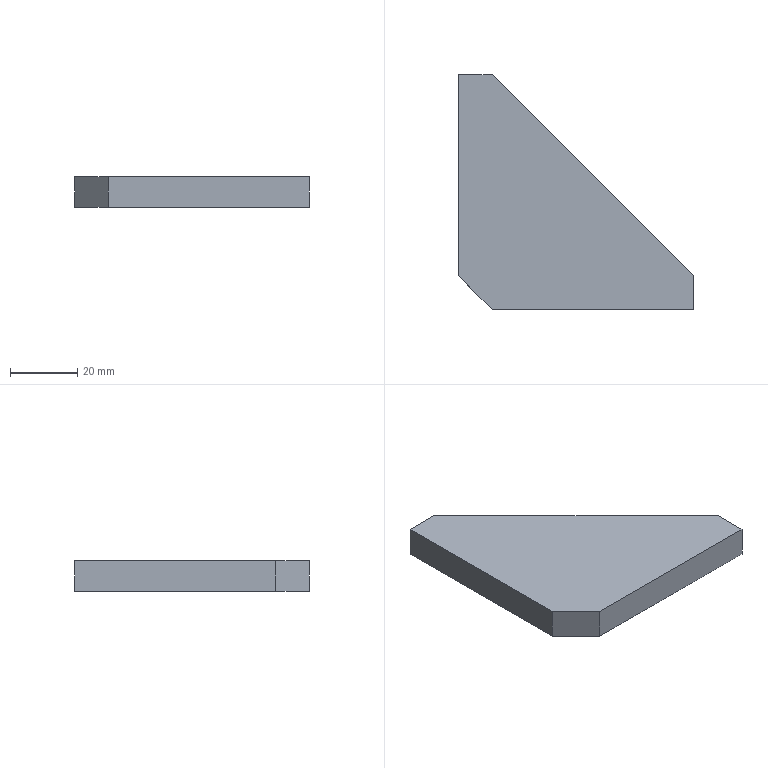Part | SolidWorks | features FlatPattern 1, SMBaseFlange 1, SheetMetal 1 | 1 solid | 8 faces | box 70 x 70 x 9 mm | volume 27450 mm3 | plane 8
STEP:
#1=CARTESIAN_POINT('',(489.387,-110.303,0.));
#2=VERTEX_POINT('',#1);
#3=CARTESIAN_POINT('',(489.387,-100.303,0.));
#4=VERTEX_POINT('',#3);
#5=CARTESIAN_POINT('',(489.387,-110.303,0.));
#6=DIRECTION('',(0.,1.,0.));
#7=VECTOR('',#6,1000.);
#8=LINE('',#5,#7);
#9=EDGE_CURVE('',#2,#4,#8,.T.);
#10=ORIENTED_EDGE('',*,*,#9,.F.);
#11=CARTESIAN_POINT('',(489.387,-110.303,-9.));
#12=VERTEX_POINT('',#11);
#13=CARTESIAN_POINT('',(489.387,-110.303,-9.));
#14=DIRECTION('',(0.,0.,1.));
#15=VECTOR('',#14,1000.);
#16=LINE('',#13,#15);
#17=EDGE_CURVE('',#12,#2,#16,.T.);
#18=ORIENTED_EDGE('',*,*,#17,.F.);
#19=CARTESIAN_POINT('',(489.387,-100.303,-9.));
#20=VERTEX_POINT('',#19);
#21=CARTESIAN_POINT('',(489.387,-110.303,-9.));
#22=DIRECTION('',(0.,1.,0.));
#23=VECTOR('',#22,1000.);
#24=LINE('',#21,#23);
#25=EDGE_CURVE('',#12,#20,#24,.T.);
#26=ORIENTED_EDGE('',*,*,#25,.T.);
#27=CARTESIAN_POINT('',(489.387,-100.303,-9.));
#28=DIRECTION('',(0.,0.,1.));
#29=VECTOR('',#28,1000.);
#30=LINE('',#27,#29);
#31=EDGE_CURVE('',#20,#4,#30,.T.);
#32=ORIENTED_EDGE('',*,*,#31,.T.);
#33=EDGE_LOOP('',(#10,#18,#26,#32));
#34=FACE_OUTER_BOUND('',#33,.T.);
#35=CARTESIAN_POINT('',(489.387,-110.303,-9.));
#36=DIRECTION('',(1.,0.,0.));
#37=DIRECTION('',(0.,0.,-1.));
#38=AXIS2_PLACEMENT_3D('',#35,#36,#37);
#39=PLANE('',#38);
#40=ADVANCED_FACE('',(#34),#39,.T.);
#41=CARTESIAN_POINT('',(429.387,-110.303,0.));
#42=VERTEX_POINT('',#41);
#43=CARTESIAN_POINT('',(429.387,-110.303,0.));
#44=DIRECTION('',(1.,0.,0.));
#45=VECTOR('',#44,1000.);
#46=LINE('',#43,#45);
#47=EDGE_CURVE('',#42,#2,#46,.T.);
#48=ORIENTED_EDGE('',*,*,#47,.F.);
#49=CARTESIAN_POINT('',(429.387,-110.303,-9.));
#50=VERTEX_POINT('',#49);
#51=CARTESIAN_POINT('',(429.387,-110.303,-9.));
#52=DIRECTION('',(0.,0.,1.));
#53=VECTOR('',#52,1000.);
#54=LINE('',#51,#53);
#55=EDGE_CURVE('',#50,#42,#54,.T.);
#56=ORIENTED_EDGE('',*,*,#55,.F.);
#57=CARTESIAN_POINT('',(429.387,-110.303,-9.));
#58=DIRECTION('',(1.,0.,0.));
#59=VECTOR('',#58,1000.);
#60=LINE('',#57,#59);
#61=EDGE_CURVE('',#50,#12,#60,.T.);
#62=ORIENTED_EDGE('',*,*,#61,.T.);
#63=ORIENTED_EDGE('',*,*,#17,.T.);
#64=EDGE_LOOP('',(#48,#56,#62,#63));
#65=FACE_OUTER_BOUND('',#64,.T.);
#66=CARTESIAN_POINT('',(429.387,-110.303,-9.));
#67=DIRECTION('',(0.,-1.,0.));
#68=DIRECTION('',(1.,0.,0.));
#69=AXIS2_PLACEMENT_3D('',#66,#67,#68);
#70=PLANE('',#69);
#71=ADVANCED_FACE('',(#65),#70,.T.);
#72=CARTESIAN_POINT('',(419.387,-100.303,0.));
#73=VERTEX_POINT('',#72);
#74=CARTESIAN_POINT('',(419.387,-100.303,0.));
#75=DIRECTION('',(0.7071,-0.7071,0.));
#76=VECTOR('',#75,1000.);
#77=LINE('',#74,#76);
#78=EDGE_CURVE('',#73,#42,#77,.T.);
#79=ORIENTED_EDGE('',*,*,#78,.F.);
#80=CARTESIAN_POINT('',(419.387,-100.303,-9.));
#81=VERTEX_POINT('',#80);
#82=CARTESIAN_POINT('',(419.387,-100.303,-9.));
#83=DIRECTION('',(0.,0.,1.));
#84=VECTOR('',#83,1000.);
#85=LINE('',#82,#84);
#86=EDGE_CURVE('',#81,#73,#85,.T.);
#87=ORIENTED_EDGE('',*,*,#86,.F.);
#88=CARTESIAN_POINT('',(419.387,-100.303,-9.));
#89=DIRECTION('',(0.7071,-0.7071,0.));
#90=VECTOR('',#89,1000.);
#91=LINE('',#88,#90);
#92=EDGE_CURVE('',#81,#50,#91,.T.);
#93=ORIENTED_EDGE('',*,*,#92,.T.);
#94=ORIENTED_EDGE('',*,*,#55,.T.);
#95=EDGE_LOOP('',(#79,#87,#93,#94));
#96=FACE_OUTER_BOUND('',#95,.T.);
#97=CARTESIAN_POINT('',(419.387,-100.303,-9.));
#98=DIRECTION('',(-0.7071,-0.7071,0.));
#99=DIRECTION('',(0.7071,-0.7071,0.));
#100=AXIS2_PLACEMENT_3D('',#97,#98,#99);
#101=PLANE('',#100);
#102=ADVANCED_FACE('',(#96),#101,.T.);
#103=CARTESIAN_POINT('',(419.387,-40.303,0.));
#104=VERTEX_POINT('',#103);
#105=CARTESIAN_POINT('',(419.387,-40.303,0.));
#106=DIRECTION('',(0.,-1.,0.));
#107=VECTOR('',#106,1000.);
#108=LINE('',#105,#107);
#109=EDGE_CURVE('',#104,#73,#108,.T.);
#110=ORIENTED_EDGE('',*,*,#109,.F.);
#111=CARTESIAN_POINT('',(419.387,-40.303,-9.));
#112=VERTEX_POINT('',#111);
#113=CARTESIAN_POINT('',(419.387,-40.303,-9.));
#114=DIRECTION('',(0.,0.,1.));
#115=VECTOR('',#114,1000.);
#116=LINE('',#113,#115);
#117=EDGE_CURVE('',#112,#104,#116,.T.);
#118=ORIENTED_EDGE('',*,*,#117,.F.);
#119=CARTESIAN_POINT('',(419.387,-40.303,-9.));
#120=DIRECTION('',(0.,-1.,0.));
#121=VECTOR('',#120,1000.);
#122=LINE('',#119,#121);
#123=EDGE_CURVE('',#112,#81,#122,.T.);
#124=ORIENTED_EDGE('',*,*,#123,.T.);
#125=ORIENTED_EDGE('',*,*,#86,.T.);
#126=EDGE_LOOP('',(#110,#118,#124,#125));
#127=FACE_OUTER_BOUND('',#126,.T.);
#128=CARTESIAN_POINT('',(419.387,-40.303,-9.));
#129=DIRECTION('',(-1.,0.,0.));
#130=DIRECTION('',(0.,0.,1.));
#131=AXIS2_PLACEMENT_3D('',#128,#129,#130);
#132=PLANE('',#131);
#133=ADVANCED_FACE('',(#127),#132,.T.);
#134=CARTESIAN_POINT('',(429.387,-40.303,0.));
#135=VERTEX_POINT('',#134);
#136=CARTESIAN_POINT('',(429.387,-40.303,0.));
#137=DIRECTION('',(-1.,0.,0.));
#138=VECTOR('',#137,1000.);
#139=LINE('',#136,#138);
#140=EDGE_CURVE('',#135,#104,#139,.T.);
#141=ORIENTED_EDGE('',*,*,#140,.F.);
#142=CARTESIAN_POINT('',(429.387,-40.303,-9.));
#143=VERTEX_POINT('',#142);
#144=CARTESIAN_POINT('',(429.387,-40.303,-9.));
#145=DIRECTION('',(0.,0.,1.));
#146=VECTOR('',#145,1000.);
#147=LINE('',#144,#146);
#148=EDGE_CURVE('',#143,#135,#147,.T.);
#149=ORIENTED_EDGE('',*,*,#148,.F.);
#150=CARTESIAN_POINT('',(429.387,-40.303,-9.));
#151=DIRECTION('',(-1.,0.,0.));
#152=VECTOR('',#151,1000.);
#153=LINE('',#150,#152);
#154=EDGE_CURVE('',#143,#112,#153,.T.);
#155=ORIENTED_EDGE('',*,*,#154,.T.);
#156=ORIENTED_EDGE('',*,*,#117,.T.);
#157=EDGE_LOOP('',(#141,#149,#155,#156));
#158=FACE_OUTER_BOUND('',#157,.T.);
#159=CARTESIAN_POINT('',(429.387,-40.303,-9.));
#160=DIRECTION('',(0.,1.,0.));
#161=DIRECTION('',(0.,0.,1.));
#162=AXIS2_PLACEMENT_3D('',#159,#160,#161);
#163=PLANE('',#162);
#164=ADVANCED_FACE('',(#158),#163,.T.);
#165=CARTESIAN_POINT('',(489.387,-100.303,0.));
#166=DIRECTION('',(-0.7071,0.7071,0.));
#167=VECTOR('',#166,1000.);
#168=LINE('',#165,#167);
#169=EDGE_CURVE('',#4,#135,#168,.T.);
#170=ORIENTED_EDGE('',*,*,#169,.F.);
#171=ORIENTED_EDGE('',*,*,#31,.F.);
#172=CARTESIAN_POINT('',(489.387,-100.303,-9.));
#173=DIRECTION('',(-0.7071,0.7071,0.));
#174=VECTOR('',#173,1000.);
#175=LINE('',#172,#174);
#176=EDGE_CURVE('',#20,#143,#175,.T.);
#177=ORIENTED_EDGE('',*,*,#176,.T.);
#178=ORIENTED_EDGE('',*,*,#148,.T.);
#179=EDGE_LOOP('',(#170,#171,#177,#178));
#180=FACE_OUTER_BOUND('',#179,.T.);
#181=CARTESIAN_POINT('',(489.387,-100.303,-9.));
#182=DIRECTION('',(0.7071,0.7071,0.));
#183=DIRECTION('',(-0.7071,0.7071,0.));
#184=AXIS2_PLACEMENT_3D('',#181,#182,#183);
#185=PLANE('',#184);
#186=ADVANCED_FACE('',(#180),#185,.T.);
#187=ORIENTED_EDGE('',*,*,#25,.F.);
#188=ORIENTED_EDGE('',*,*,#61,.F.);
#189=ORIENTED_EDGE('',*,*,#92,.F.);
#190=ORIENTED_EDGE('',*,*,#123,.F.);
#191=ORIENTED_EDGE('',*,*,#154,.F.);
#192=ORIENTED_EDGE('',*,*,#176,.F.);
#193=EDGE_LOOP('',(#187,#188,#189,#190,#191,#192));
#194=FACE_OUTER_BOUND('',#193,.T.);
#195=CARTESIAN_POINT('',(0.,0.,-9.));
#196=DIRECTION('',(0.,0.,1.));
#197=DIRECTION('',(1.,0.,0.));
#198=AXIS2_PLACEMENT_3D('',#195,#196,#197);
#199=PLANE('',#198);
#200=ADVANCED_FACE('',(#194),#199,.F.);
#201=ORIENTED_EDGE('',*,*,#9,.T.);
#202=ORIENTED_EDGE('',*,*,#169,.T.);
#203=ORIENTED_EDGE('',*,*,#140,.T.);
#204=ORIENTED_EDGE('',*,*,#109,.T.);
#205=ORIENTED_EDGE('',*,*,#78,.T.);
#206=ORIENTED_EDGE('',*,*,#47,.T.);
#207=EDGE_LOOP('',(#201,#202,#203,#204,#205,#206));
#208=FACE_OUTER_BOUND('',#207,.T.);
#209=CARTESIAN_POINT('',(0.,0.,0.));
#210=DIRECTION('',(0.,0.,1.));
#211=DIRECTION('',(1.,0.,0.));
#212=AXIS2_PLACEMENT_3D('',#209,#210,#211);
#213=PLANE('',#212);
#214=ADVANCED_FACE('',(#208),#213,.T.);
#215=CLOSED_SHELL('',(#40,#71,#102,#133,#164,#186,#200,#214));
#216=MANIFOLD_SOLID_BREP('',#215);
#217=CARTESIAN_POINT('',(0.,0.,0.));
#218=DIRECTION('',(0.,0.,1.));
#219=DIRECTION('',(1.,0.,0.));
#220=AXIS2_PLACEMENT_3D('',#217,#218,#219);
#221=(LENGTH_UNIT()NAMED_UNIT(*)SI_UNIT(.MILLI.,.METRE.));
#222=UNCERTAINTY_MEASURE_WITH_UNIT(LENGTH_MEASURE(0.00001),#221,'','');
#223=(NAMED_UNIT(*)PLANE_ANGLE_UNIT()SI_UNIT($,.RADIAN.));
#224=(NAMED_UNIT(*)SI_UNIT($,.STERADIAN.)SOLID_ANGLE_UNIT());
#225=(GEOMETRIC_REPRESENTATION_CONTEXT(3)GLOBAL_UNCERTAINTY_ASSIGNED_CONTEXT((#222))GLOBAL_UNIT_ASSIGNED_CONTEXT((#221,#223,#224))REPRESENTATION_CONTEXT('',''));
#226=ADVANCED_BREP_SHAPE_REPRESENTATION('',(#216,#220),#225);